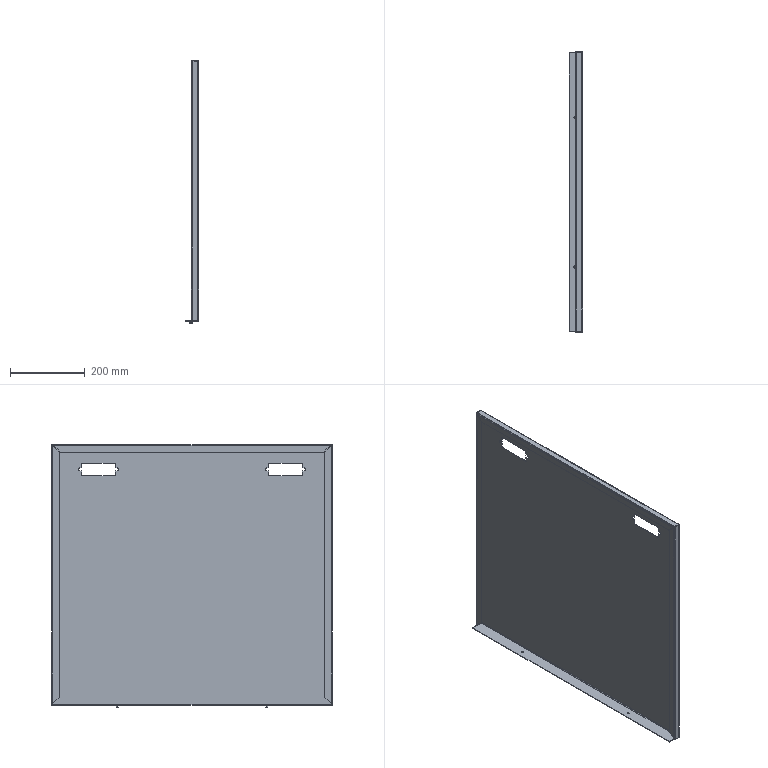Part | STEP file | PRT0544B_HI-003_B-2 | 3 solids | 94 faces | box 35 x 750 x 702 mm | volume 920814 mm3 | plane 62 | cylinder 26 | spline 6 | commonest cylinder face diameters 3 x11 6 x11 8 x4